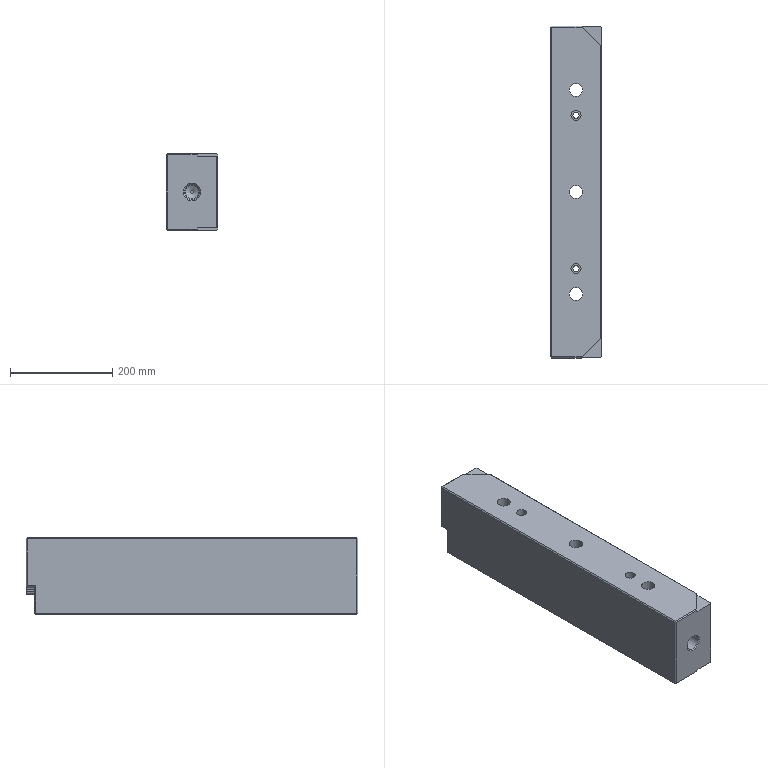Part | STEP file | SOLID | 1 solid | 193 faces | box 100 x 650 x 150 mm | volume 9243091 mm3 | plane 99 | cylinder 39 | cone 37 | other 18 | commonest cylinder face diameters 14 x4 15.947 x4 16 x4 20 x4 26 x3 3.333 x2